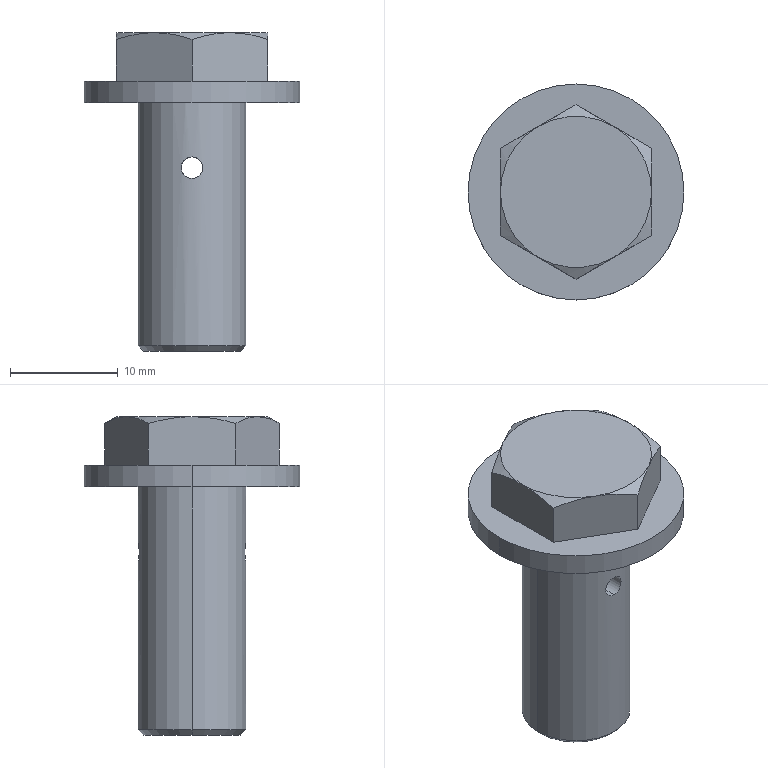Part | SolidWorks | features BaseBody 1 | 1 solid | 31 faces | box 20 x 20 x 29.5 mm | volume 2987 mm3 | plane 11 | cylinder 10 | cone 10 | commonest cylinder face diameters 2 x4 3.5 x2 10 x2 20 x2
STEP:
#1=CARTESIAN_POINT('',(135.5,59.,62.5));
#2=VERTEX_POINT('',#1);
#3=CARTESIAN_POINT('',(155.5,59.,62.5));
#4=VERTEX_POINT('',#3);
#5=CARTESIAN_POINT('',(145.5,59.,62.5));
#6=DIRECTION('',(0.,0.,-1.));
#7=DIRECTION('',(-1.,0.,0.));
#8=AXIS2_PLACEMENT_3D('',#5,#6,#7);
#9=CIRCLE('',#8,10.);
#10=EDGE_CURVE('',#2,#4,#9,.T.);
#11=ORIENTED_EDGE('',*,*,#10,.T.);
#12=CARTESIAN_POINT('',(155.5,59.,60.5));
#13=VERTEX_POINT('',#12);
#14=CARTESIAN_POINT('',(155.5,59.,62.5));
#15=DIRECTION('',(0.,0.,-1.));
#16=VECTOR('',#15,1000.);
#17=LINE('',#14,#16);
#18=EDGE_CURVE('',#4,#13,#17,.T.);
#19=ORIENTED_EDGE('',*,*,#18,.T.);
#20=CARTESIAN_POINT('',(135.5,59.,60.5));
#21=VERTEX_POINT('',#20);
#22=CARTESIAN_POINT('',(145.5,59.,60.5));
#23=DIRECTION('',(0.,0.,-1.));
#24=DIRECTION('',(-1.,0.,0.));
#25=AXIS2_PLACEMENT_3D('',#22,#23,#24);
#26=CIRCLE('',#25,10.);
#27=EDGE_CURVE('',#21,#13,#26,.T.);
#28=ORIENTED_EDGE('',*,*,#27,.F.);
#29=CARTESIAN_POINT('',(135.5,59.,62.5));
#30=DIRECTION('',(0.,0.,-1.));
#31=VECTOR('',#30,1000.);
#32=LINE('',#29,#31);
#33=EDGE_CURVE('',#2,#21,#32,.T.);
#34=ORIENTED_EDGE('',*,*,#33,.F.);
#35=EDGE_LOOP('',(#11,#19,#28,#34));
#36=FACE_OUTER_BOUND('',#35,.T.);
#37=CARTESIAN_POINT('',(145.5,59.,62.5));
#38=DIRECTION('',(0.,0.,-1.));
#39=DIRECTION('',(-1.,0.,0.));
#40=AXIS2_PLACEMENT_3D('',#37,#38,#39);
#41=CYLINDRICAL_SURFACE('',#40,10.);
#42=ADVANCED_FACE('',(#36),#41,.T.);
#43=CARTESIAN_POINT('',(145.5,54.,55.5));
#44=VERTEX_POINT('',#43);
#45=CARTESIAN_POINT('',(145.5,54.,53.5));
#46=VERTEX_POINT('',#45);
#47=CARTESIAN_POINT('',(145.5,54.,55.5));
#48=CARTESIAN_POINT('',(145.631,54.,55.5));
#49=CARTESIAN_POINT('',(145.763,54.005,55.474));
#50=CARTESIAN_POINT('',(146.003,54.024,55.374));
#51=CARTESIAN_POINT('',(146.114,54.037,55.3));
#52=CARTESIAN_POINT('',(146.299,54.063,55.115));
#53=CARTESIAN_POINT('',(146.373,54.077,55.005));
#54=CARTESIAN_POINT('',(146.474,54.095,54.763));
#55=CARTESIAN_POINT('',(146.5,54.101,54.633));
#56=CARTESIAN_POINT('',(146.5,54.101,54.368));
#57=CARTESIAN_POINT('',(146.474,54.095,54.238));
#58=CARTESIAN_POINT('',(146.374,54.077,53.996));
#59=CARTESIAN_POINT('',(146.299,54.063,53.885));
#60=CARTESIAN_POINT('',(146.116,54.037,53.701));
#61=CARTESIAN_POINT('',(146.004,54.024,53.627));
#62=CARTESIAN_POINT('',(145.764,54.006,53.527));
#63=CARTESIAN_POINT('',(145.632,54.,53.5));
#64=CARTESIAN_POINT('',(145.5,54.,53.5));
#65=B_SPLINE_CURVE_WITH_KNOTS('',3,(#47,#48,#49,#50,#51,#52,#53,#54,#55,#56,#57,#58,#59,#60,#61,#62,#63,#64),.UNSPECIFIED.,.F.,.F.,(4,2,2,2,2,2,2,2,4),(0.003134,0.003526,0.003918,0.004309,0.004701,0.005093,0.005485,0.005876,0.006268),.UNSPECIFIED.);
#66=EDGE_CURVE('',#44,#46,#65,.T.);
#67=ORIENTED_EDGE('',*,*,#66,.F.);
#68=CARTESIAN_POINT('',(145.5,57.25,55.5));
#69=VERTEX_POINT('',#68);
#70=CARTESIAN_POINT('',(145.5,50.917,55.5));
#71=DIRECTION('',(0.,1.,0.));
#72=VECTOR('',#71,1000.);
#73=LINE('',#70,#72);
#74=EDGE_CURVE('',#44,#69,#73,.T.);
#75=ORIENTED_EDGE('',*,*,#74,.T.);
#76=CARTESIAN_POINT('',(145.5,57.25,53.5));
#77=VERTEX_POINT('',#76);
#78=CARTESIAN_POINT('',(145.5,57.25,53.5));
#79=CARTESIAN_POINT('',(145.635,57.25,53.5));
#80=CARTESIAN_POINT('',(145.768,57.266,53.528));
#81=CARTESIAN_POINT('',(146.009,57.321,53.63));
#82=CARTESIAN_POINT('',(146.118,57.36,53.704));
#83=CARTESIAN_POINT('',(146.298,57.44,53.884));
#84=CARTESIAN_POINT('',(146.371,57.481,53.992));
#85=CARTESIAN_POINT('',(146.472,57.543,54.231));
#86=CARTESIAN_POINT('',(146.5,57.564,54.364));
#87=CARTESIAN_POINT('',(146.5,57.564,54.635));
#88=CARTESIAN_POINT('',(146.472,57.544,54.768));
#89=CARTESIAN_POINT('',(146.371,57.481,55.008));
#90=CARTESIAN_POINT('',(146.298,57.439,55.116));
#91=CARTESIAN_POINT('',(146.117,57.36,55.297));
#92=CARTESIAN_POINT('',(146.009,57.321,55.37));
#93=CARTESIAN_POINT('',(145.767,57.266,55.472));
#94=CARTESIAN_POINT('',(145.636,57.25,55.5));
#95=CARTESIAN_POINT('',(145.5,57.25,55.5));
#96=B_SPLINE_CURVE_WITH_KNOTS('',3,(#78,#79,#80,#81,#82,#83,#84,#85,#86,#87,#88,#89,#90,#91,#92,#93,#94,#95),.UNSPECIFIED.,.F.,.F.,(4,2,2,2,2,2,2,2,4),(0.,0.0003999,0.0007999,0.0012,0.0016,0.002,0.0024,0.0028,0.003199),.UNSPECIFIED.);
#97=EDGE_CURVE('',#77,#69,#96,.T.);
#98=ORIENTED_EDGE('',*,*,#97,.F.);
#99=CARTESIAN_POINT('',(145.5,50.917,53.5));
#100=DIRECTION('',(0.,1.,0.));
#101=VECTOR('',#100,1000.);
#102=LINE('',#99,#101);
#103=EDGE_CURVE('',#46,#77,#102,.T.);
#104=ORIENTED_EDGE('',*,*,#103,.F.);
#105=EDGE_LOOP('',(#67,#75,#98,#104));
#106=FACE_OUTER_BOUND('',#105,.T.);
#107=CARTESIAN_POINT('',(145.5,50.917,54.5));
#108=DIRECTION('',(0.,1.,0.));
#109=DIRECTION('',(0.,0.,-1.));
#110=AXIS2_PLACEMENT_3D('',#107,#108,#109);
#111=CYLINDRICAL_SURFACE('',#110,1.);
#112=ADVANCED_FACE('',(#106),#111,.F.);
#113=CARTESIAN_POINT('',(145.5,60.75,55.5));
#114=VERTEX_POINT('',#113);
#115=CARTESIAN_POINT('',(145.5,60.75,53.5));
#116=VERTEX_POINT('',#115);
#117=CARTESIAN_POINT('',(145.5,60.75,55.5));
#118=CARTESIAN_POINT('',(145.635,60.75,55.5));
#119=CARTESIAN_POINT('',(145.768,60.734,55.472));
#120=CARTESIAN_POINT('',(146.009,60.679,55.371));
#121=CARTESIAN_POINT('',(146.118,60.64,55.297));
#122=CARTESIAN_POINT('',(146.298,60.561,55.116));
#123=CARTESIAN_POINT('',(146.371,60.519,55.008));
#124=CARTESIAN_POINT('',(146.472,60.457,54.769));
#125=CARTESIAN_POINT('',(146.5,60.436,54.635));
#126=CARTESIAN_POINT('',(146.5,60.436,54.366));
#127=CARTESIAN_POINT('',(146.472,60.456,54.233));
#128=CARTESIAN_POINT('',(146.372,60.519,53.993));
#129=CARTESIAN_POINT('',(146.299,60.56,53.885));
#130=CARTESIAN_POINT('',(146.118,60.64,53.703));
#131=CARTESIAN_POINT('',(146.011,60.678,53.63));
#132=CARTESIAN_POINT('',(145.768,60.734,53.528));
#133=CARTESIAN_POINT('',(145.635,60.75,53.5));
#134=CARTESIAN_POINT('',(145.5,60.75,53.5));
#135=B_SPLINE_CURVE_WITH_KNOTS('',3,(#117,#118,#119,#120,#121,#122,#123,#124,#125,#126,#127,#128,#129,#130,#131,#132,#133,#134),.UNSPECIFIED.,.F.,.F.,(4,2,2,2,2,2,2,2,4),(0.003199,0.003599,0.003998,0.004397,0.004796,0.005195,0.005594,0.005993,0.006392),.UNSPECIFIED.);
#136=EDGE_CURVE('',#114,#116,#135,.T.);
#137=ORIENTED_EDGE('',*,*,#136,.F.);
#138=CARTESIAN_POINT('',(145.5,64.,55.5));
#139=VERTEX_POINT('',#138);
#140=CARTESIAN_POINT('',(145.5,50.917,55.5));
#141=DIRECTION('',(0.,1.,0.));
#142=VECTOR('',#141,1000.);
#143=LINE('',#140,#142);
#144=EDGE_CURVE('',#114,#139,#143,.T.);
#145=ORIENTED_EDGE('',*,*,#144,.T.);
#146=CARTESIAN_POINT('',(145.5,64.,53.5));
#147=VERTEX_POINT('',#146);
#148=CARTESIAN_POINT('',(145.5,64.,53.5));
#149=CARTESIAN_POINT('',(145.633,64.,53.5));
#150=CARTESIAN_POINT('',(145.763,63.995,53.526));
#151=CARTESIAN_POINT('',(146.005,63.976,53.627));
#152=CARTESIAN_POINT('',(146.115,63.963,53.701));
#153=CARTESIAN_POINT('',(146.299,63.937,53.885));
#154=CARTESIAN_POINT('',(146.374,63.923,53.996));
#155=CARTESIAN_POINT('',(146.474,63.905,54.237));
#156=CARTESIAN_POINT('',(146.5,63.899,54.369));
#157=CARTESIAN_POINT('',(146.5,63.899,54.63));
#158=CARTESIAN_POINT('',(146.474,63.904,54.762));
#159=CARTESIAN_POINT('',(146.374,63.923,55.004));
#160=CARTESIAN_POINT('',(146.3,63.936,55.114));
#161=CARTESIAN_POINT('',(146.114,63.963,55.3));
#162=CARTESIAN_POINT('',(146.004,63.976,55.374));
#163=CARTESIAN_POINT('',(145.762,63.995,55.474));
#164=CARTESIAN_POINT('',(145.631,64.,55.5));
#165=CARTESIAN_POINT('',(145.5,64.,55.5));
#166=B_SPLINE_CURVE_WITH_KNOTS('',3,(#148,#149,#150,#151,#152,#153,#154,#155,#156,#157,#158,#159,#160,#161,#162,#163,#164,#165),.UNSPECIFIED.,.F.,.F.,(4,2,2,2,2,2,2,2,4),(0.,0.0003918,0.0007836,0.001175,0.001567,0.001959,0.002351,0.002743,0.003134),.UNSPECIFIED.);
#167=EDGE_CURVE('',#147,#139,#166,.T.);
#168=ORIENTED_EDGE('',*,*,#167,.F.);
#169=CARTESIAN_POINT('',(145.5,50.917,53.5));
#170=DIRECTION('',(0.,1.,0.));
#171=VECTOR('',#170,1000.);
#172=LINE('',#169,#171);
#173=EDGE_CURVE('',#116,#147,#172,.T.);
#174=ORIENTED_EDGE('',*,*,#173,.F.);
#175=EDGE_LOOP('',(#137,#145,#168,#174));
#176=FACE_OUTER_BOUND('',#175,.T.);
#177=CARTESIAN_POINT('',(145.5,50.917,54.5));
#178=DIRECTION('',(0.,1.,0.));
#179=DIRECTION('',(0.,0.,-1.));
#180=AXIS2_PLACEMENT_3D('',#177,#178,#179);
#181=CYLINDRICAL_SURFACE('',#180,1.);
#182=ADVANCED_FACE('',(#176),#181,.F.);
#183=CARTESIAN_POINT('',(147.25,59.,38.));
#184=VERTEX_POINT('',#183);
#185=CARTESIAN_POINT('',(143.75,59.,38.));
#186=VERTEX_POINT('',#185);
#187=CARTESIAN_POINT('',(145.5,59.,38.));
#188=DIRECTION('',(0.,0.,-1.));
#189=DIRECTION('',(-1.,0.,0.));
#190=AXIS2_PLACEMENT_3D('',#187,#188,#189);
#191=CIRCLE('',#190,1.75);
#192=EDGE_CURVE('',#184,#186,#191,.T.);
#193=ORIENTED_EDGE('',*,*,#192,.F.);
#194=CARTESIAN_POINT('',(147.75,59.,37.5));
#195=VERTEX_POINT('',#194);
#196=CARTESIAN_POINT('',(147.25,59.,38.));
#197=DIRECTION('',(0.7071,0.,-0.7071));
#198=VECTOR('',#197,1000.);
#199=LINE('',#196,#198);
#200=EDGE_CURVE('',#184,#195,#199,.T.);
#201=ORIENTED_EDGE('',*,*,#200,.T.);
#202=CARTESIAN_POINT('',(143.25,59.,37.5));
#203=VERTEX_POINT('',#202);
#204=CARTESIAN_POINT('',(145.5,59.,37.5));
#205=DIRECTION('',(0.,0.,1.));
#206=DIRECTION('',(-1.,0.,0.));
#207=AXIS2_PLACEMENT_3D('',#204,#205,#206);
#208=CIRCLE('',#207,2.25);
#209=EDGE_CURVE('',#203,#195,#208,.T.);
#210=ORIENTED_EDGE('',*,*,#209,.F.);
#211=CARTESIAN_POINT('',(143.75,59.,38.));
#212=DIRECTION('',(-0.7071,0.,-0.7071));
#213=VECTOR('',#212,1000.);
#214=LINE('',#211,#213);
#215=EDGE_CURVE('',#186,#203,#214,.T.);
#216=ORIENTED_EDGE('',*,*,#215,.F.);
#217=EDGE_LOOP('',(#193,#201,#210,#216));
#218=FACE_OUTER_BOUND('',#217,.T.);
#219=CARTESIAN_POINT('',(145.5,59.,38.));
#220=DIRECTION('',(0.,0.,-1.));
#221=DIRECTION('',(-1.,0.,0.));
#222=AXIS2_PLACEMENT_3D('',#219,#220,#221);
#223=CONICAL_SURFACE('',#222,1.75,0.7854);
#224=ADVANCED_FACE('',(#218),#223,.F.);
#225=CARTESIAN_POINT('',(141.,59.,37.5));
#226=VERTEX_POINT('',#225);
#227=CARTESIAN_POINT('',(150.,59.,37.5));
#228=VERTEX_POINT('',#227);
#229=CARTESIAN_POINT('',(145.5,59.,37.5));
#230=DIRECTION('',(0.,0.,-1.));
#231=DIRECTION('',(-1.,0.,0.));
#232=AXIS2_PLACEMENT_3D('',#229,#230,#231);
#233=CIRCLE('',#232,4.5);
#234=EDGE_CURVE('',#226,#228,#233,.T.);
#235=ORIENTED_EDGE('',*,*,#234,.F.);
#236=CARTESIAN_POINT('',(140.5,59.,38.));
#237=VERTEX_POINT('',#236);
#238=CARTESIAN_POINT('',(141.,59.,37.5));
#239=DIRECTION('',(-0.7071,0.,0.7071));
#240=VECTOR('',#239,1000.);
#241=LINE('',#238,#240);
#242=EDGE_CURVE('',#226,#237,#241,.T.);
#243=ORIENTED_EDGE('',*,*,#242,.T.);
#244=CARTESIAN_POINT('',(150.5,59.,38.));
#245=VERTEX_POINT('',#244);
#246=CARTESIAN_POINT('',(145.5,59.,38.));
#247=DIRECTION('',(0.,0.,1.));
#248=DIRECTION('',(-1.,0.,0.));
#249=AXIS2_PLACEMENT_3D('',#246,#247,#248);
#250=CIRCLE('',#249,5.);
#251=EDGE_CURVE('',#245,#237,#250,.T.);
#252=ORIENTED_EDGE('',*,*,#251,.F.);
#253=CARTESIAN_POINT('',(150.,59.,37.5));
#254=DIRECTION('',(0.7071,0.,0.7071));
#255=VECTOR('',#254,1000.);
#256=LINE('',#253,#255);
#257=EDGE_CURVE('',#228,#245,#256,.T.);
#258=ORIENTED_EDGE('',*,*,#257,.F.);
#259=EDGE_LOOP('',(#235,#243,#252,#258));
#260=FACE_OUTER_BOUND('',#259,.T.);
#261=CARTESIAN_POINT('',(145.5,59.,37.5));
#262=DIRECTION('',(0.,0.,1.));
#263=DIRECTION('',(1.,0.,0.));
#264=AXIS2_PLACEMENT_3D('',#261,#262,#263);
#265=CONICAL_SURFACE('',#264,4.5,0.7854);
#266=ADVANCED_FACE('',(#260),#265,.T.);
#267=ORIENTED_EDGE('',*,*,#97,.T.);
#268=CARTESIAN_POINT('',(145.5,57.25,55.5));
#269=CARTESIAN_POINT('',(145.365,57.25,55.5));
#270=CARTESIAN_POINT('',(145.232,57.266,55.472));
#271=CARTESIAN_POINT('',(144.991,57.321,55.371));
#272=CARTESIAN_POINT('',(144.882,57.36,55.297));
#273=CARTESIAN_POINT('',(144.702,57.439,55.116));
#274=CARTESIAN_POINT('',(144.629,57.481,55.008));
#275=CARTESIAN_POINT('',(144.528,57.543,54.769));
#276=CARTESIAN_POINT('',(144.5,57.564,54.635));
#277=CARTESIAN_POINT('',(144.5,57.564,54.366));
#278=CARTESIAN_POINT('',(144.528,57.544,54.233));
#279=CARTESIAN_POINT('',(144.628,57.481,53.993));
#280=CARTESIAN_POINT('',(144.701,57.44,53.885));
#281=CARTESIAN_POINT('',(144.882,57.36,53.703));
#282=CARTESIAN_POINT('',(144.989,57.322,53.63));
#283=CARTESIAN_POINT('',(145.232,57.266,53.528));
#284=CARTESIAN_POINT('',(145.365,57.25,53.5));
#285=CARTESIAN_POINT('',(145.5,57.25,53.5));
#286=B_SPLINE_CURVE_WITH_KNOTS('',3,(#268,#269,#270,#271,#272,#273,#274,#275,#276,#277,#278,#279,#280,#281,#282,#283,#284,#285),.UNSPECIFIED.,.F.,.F.,(4,2,2,2,2,2,2,2,4),(0.003199,0.003599,0.003998,0.004397,0.004796,0.005195,0.005594,0.005993,0.006392),.UNSPECIFIED.);
#287=EDGE_CURVE('',#69,#77,#286,.T.);
#288=ORIENTED_EDGE('',*,*,#287,.T.);
#289=EDGE_LOOP('',(#267,#288));
#290=FACE_BOUND('',#289,.T.);
#291=CARTESIAN_POINT('',(147.25,59.,56.5));
#292=VERTEX_POINT('',#291);
#293=CARTESIAN_POINT('',(143.75,59.,56.5));
#294=VERTEX_POINT('',#293);
#295=CARTESIAN_POINT('',(145.5,59.,56.5));
#296=DIRECTION('',(0.,0.,-1.));
#297=DIRECTION('',(-1.,0.,0.));
#298=AXIS2_PLACEMENT_3D('',#295,#296,#297);
#299=CIRCLE('',#298,1.75);
#300=EDGE_CURVE('',#292,#294,#299,.T.);
#301=ORIENTED_EDGE('',*,*,#300,.F.);
#302=CARTESIAN_POINT('',(147.25,59.,56.5));
#303=DIRECTION('',(0.,0.,-1.));
#304=VECTOR('',#303,1000.);
#305=LINE('',#302,#304);
#306=EDGE_CURVE('',#292,#184,#305,.T.);
#307=ORIENTED_EDGE('',*,*,#306,.T.);
#308=ORIENTED_EDGE('',*,*,#192,.T.);
#309=CARTESIAN_POINT('',(143.75,59.,56.5));
#310=DIRECTION('',(0.,0.,-1.));
#311=VECTOR('',#310,1000.);
#312=LINE('',#309,#311);
#313=EDGE_CURVE('',#294,#186,#312,.T.);
#314=ORIENTED_EDGE('',*,*,#313,.F.);
#315=EDGE_LOOP('',(#301,#307,#308,#314));
#316=FACE_OUTER_BOUND('',#315,.T.);
#317=CARTESIAN_POINT('',(145.5,59.,56.5));
#318=DIRECTION('',(0.,0.,-1.));
#319=DIRECTION('',(-1.,0.,0.));
#320=AXIS2_PLACEMENT_3D('',#317,#318,#319);
#321=CYLINDRICAL_SURFACE('',#320,1.75);
#322=ADVANCED_FACE('',(#290,#316),#321,.F.);
#323=ORIENTED_EDGE('',*,*,#167,.T.);
#324=CARTESIAN_POINT('',(145.5,64.,55.5));
#325=CARTESIAN_POINT('',(145.369,64.,55.5));
#326=CARTESIAN_POINT('',(145.237,63.995,55.474));
#327=CARTESIAN_POINT('',(144.997,63.976,55.374));
#328=CARTESIAN_POINT('',(144.886,63.963,55.3));
#329=CARTESIAN_POINT('',(144.701,63.937,55.115));
#330=CARTESIAN_POINT('',(144.627,63.923,55.005));
#331=CARTESIAN_POINT('',(144.526,63.905,54.763));
#332=CARTESIAN_POINT('',(144.5,63.899,54.633));
#333=CARTESIAN_POINT('',(144.5,63.899,54.368));
#334=CARTESIAN_POINT('',(144.526,63.905,54.238));
#335=CARTESIAN_POINT('',(144.626,63.923,53.996));
#336=CARTESIAN_POINT('',(144.701,63.937,53.885));
#337=CARTESIAN_POINT('',(144.884,63.963,53.701));
#338=CARTESIAN_POINT('',(144.996,63.976,53.627));
#339=CARTESIAN_POINT('',(145.236,63.994,53.527));
#340=CARTESIAN_POINT('',(145.368,64.,53.5));
#341=CARTESIAN_POINT('',(145.5,64.,53.5));
#342=B_SPLINE_CURVE_WITH_KNOTS('',3,(#324,#325,#326,#327,#328,#329,#330,#331,#332,#333,#334,#335,#336,#337,#338,#339,#340,#341),.UNSPECIFIED.,.F.,.F.,(4,2,2,2,2,2,2,2,4),(0.003134,0.003526,0.003918,0.004309,0.004701,0.005093,0.005485,0.005876,0.006268),.UNSPECIFIED.);
#343=EDGE_CURVE('',#139,#147,#342,.T.);
#344=ORIENTED_EDGE('',*,*,#343,.T.);
#345=EDGE_LOOP('',(#323,#344));
#346=FACE_BOUND('',#345,.T.);
#347=ORIENTED_EDGE('',*,*,#251,.T.);
#348=CARTESIAN_POINT('',(140.5,59.,60.5));
#349=VERTEX_POINT('',#348);
#350=CARTESIAN_POINT('',(140.5,59.,37.5));
#351=DIRECTION('',(0.,0.,1.));
#352=VECTOR('',#351,1000.);
#353=LINE('',#350,#352);
#354=EDGE_CURVE('',#237,#349,#353,.T.);
#355=ORIENTED_EDGE('',*,*,#354,.T.);
#356=CARTESIAN_POINT('',(150.5,59.,60.5));
#357=VERTEX_POINT('',#356);
#358=CARTESIAN_POINT('',(145.5,59.,60.5));
#359=DIRECTION('',(0.,0.,-1.));
#360=DIRECTION('',(-1.,0.,0.));
#361=AXIS2_PLACEMENT_3D('',#358,#359,#360);
#362=CIRCLE('',#361,5.);
#363=EDGE_CURVE('',#349,#357,#362,.T.);
#364=ORIENTED_EDGE('',*,*,#363,.T.);
#365=CARTESIAN_POINT('',(150.5,59.,37.5));
#366=DIRECTION('',(0.,0.,1.));
#367=VECTOR('',#366,1000.);
#368=LINE('',#365,#367);
#369=EDGE_CURVE('',#245,#357,#368,.T.);
#370=ORIENTED_EDGE('',*,*,#369,.F.);
#371=EDGE_LOOP('',(#347,#355,#364,#370));
#372=FACE_OUTER_BOUND('',#371,.T.);
#373=CARTESIAN_POINT('',(145.5,59.,37.5));
#374=DIRECTION('',(0.,0.,1.));
#375=DIRECTION('',(1.,0.,0.));
#376=AXIS2_PLACEMENT_3D('',#373,#374,#375);
#377=CYLINDRICAL_SURFACE('',#376,5.);
#378=ADVANCED_FACE('',(#346,#372),#377,.T.);
#379=CARTESIAN_POINT('',(145.5,59.,60.5));
#380=DIRECTION('',(0.,0.,-1.));
#381=DIRECTION('',(-1.,0.,0.));
#382=AXIS2_PLACEMENT_3D('',#379,#380,#381);
#383=CIRCLE('',#382,5.);
#384=EDGE_CURVE('',#357,#349,#383,.T.);
#385=ORIENTED_EDGE('',*,*,#384,.F.);
#386=ORIENTED_EDGE('',*,*,#363,.F.);
#387=EDGE_LOOP('',(#385,#386));
#388=FACE_BOUND('',#387,.T.);
#389=ORIENTED_EDGE('',*,*,#27,.T.);
#390=CARTESIAN_POINT('',(145.5,59.,60.5));
#391=DIRECTION('',(0.,0.,-1.));
#392=DIRECTION('',(-1.,0.,0.));
#393=AXIS2_PLACEMENT_3D('',#390,#391,#392);
#394=CIRCLE('',#393,10.);
#395=EDGE_CURVE('',#13,#21,#394,.T.);
#396=ORIENTED_EDGE('',*,*,#395,.T.);
#397=EDGE_LOOP('',(#389,#396));
#398=FACE_OUTER_BOUND('',#397,.T.);
#399=CARTESIAN_POINT('',(145.5,67.083,60.5));
#400=DIRECTION('',(0.,0.,-1.));
#401=DIRECTION('',(-1.,0.,0.));
#402=AXIS2_PLACEMENT_3D('',#399,#400,#401);
#403=PLANE('',#402);
#404=ADVANCED_FACE('',(#388,#398),#403,.T.);
#405=ORIENTED_EDGE('',*,*,#354,.F.);
#406=CARTESIAN_POINT('',(145.5,59.,38.));
#407=DIRECTION('',(0.,0.,1.));
#408=DIRECTION('',(-1.,0.,0.));
#409=AXIS2_PLACEMENT_3D('',#406,#407,#408);
#410=CIRCLE('',#409,5.);
#411=EDGE_CURVE('',#237,#245,#410,.T.);
#412=ORIENTED_EDGE('',*,*,#411,.T.);
#413=ORIENTED_EDGE('',*,*,#369,.T.);
#414=ORIENTED_EDGE('',*,*,#384,.T.);
#415=EDGE_LOOP('',(#405,#412,#413,#414));
#416=FACE_OUTER_BOUND('',#415,.T.);
#417=CARTESIAN_POINT('',(145.5,54.,53.5));
#418=CARTESIAN_POINT('',(145.367,54.,53.5));
#419=CARTESIAN_POINT('',(145.237,54.005,53.526));
#420=CARTESIAN_POINT('',(144.995,54.024,53.627));
#421=CARTESIAN_POINT('',(144.885,54.037,53.701));
#422=CARTESIAN_POINT('',(144.701,54.063,53.885));
#423=CARTESIAN_POINT('',(144.626,54.077,53.996));
#424=CARTESIAN_POINT('',(144.526,54.095,54.237));
#425=CARTESIAN_POINT('',(144.5,54.101,54.369));
#426=CARTESIAN_POINT('',(144.5,54.101,54.63));
#427=CARTESIAN_POINT('',(144.526,54.096,54.762));
#428=CARTESIAN_POINT('',(144.626,54.077,55.004));
#429=CARTESIAN_POINT('',(144.7,54.064,55.114));
#430=CARTESIAN_POINT('',(144.886,54.037,55.3));
#431=CARTESIAN_POINT('',(144.996,54.024,55.374));
#432=CARTESIAN_POINT('',(145.238,54.005,55.474));
#433=CARTESIAN_POINT('',(145.369,54.,55.5));
#434=CARTESIAN_POINT('',(145.5,54.,55.5));
#435=B_SPLINE_CURVE_WITH_KNOTS('',3,(#417,#418,#419,#420,#421,#422,#423,#424,#425,#426,#427,#428,#429,#430,#431,#432,#433,#434),.UNSPECIFIED.,.F.,.F.,(4,2,2,2,2,2,2,2,4),(0.,0.0003918,0.0007836,0.001175,0.001567,0.001959,0.002351,0.002743,0.003134),.UNSPECIFIED.);
#436=EDGE_CURVE('',#46,#44,#435,.T.);
#437=ORIENTED_EDGE('',*,*,#436,.T.);
#438=ORIENTED_EDGE('',*,*,#66,.T.);
#439=EDGE_LOOP('',(#437,#438));
#440=FACE_BOUND('',#439,.T.);
#441=CARTESIAN_POINT('',(145.5,59.,37.5));
#442=DIRECTION('',(0.,0.,1.));
#443=DIRECTION('',(1.,0.,0.));
#444=AXIS2_PLACEMENT_3D('',#441,#442,#443);
#445=CYLINDRICAL_SURFACE('',#444,5.);
#446=ADVANCED_FACE('',(#416,#440),#445,.T.);
#447=ORIENTED_EDGE('',*,*,#209,.T.);
#448=CARTESIAN_POINT('',(145.5,59.,37.5));
#449=DIRECTION('',(0.,0.,1.));
#450=DIRECTION('',(-1.,0.,0.));
#451=AXIS2_PLACEMENT_3D('',#448,#449,#450);
#452=CIRCLE('',#451,2.25);
#453=EDGE_CURVE('',#195,#203,#452,.T.);
#454=ORIENTED_EDGE('',*,*,#453,.T.);
#455=EDGE_LOOP('',(#447,#454));
#456=FACE_BOUND('',#455,.T.);
#457=CARTESIAN_POINT('',(145.5,59.,37.5));
#458=DIRECTION('',(0.,0.,-1.));
#459=DIRECTION('',(-1.,0.,0.));
#460=AXIS2_PLACEMENT_3D('',#457,#458,#459);
#461=CIRCLE('',#460,4.5);
#462=EDGE_CURVE('',#228,#226,#461,.T.);
#463=ORIENTED_EDGE('',*,*,#462,.T.);
#464=ORIENTED_EDGE('',*,*,#234,.T.);
#465=EDGE_LOOP('',(#463,#464));
#466=FACE_OUTER_BOUND('',#465,.T.);
#467=CARTESIAN_POINT('',(145.5,59.,37.5));
#468=DIRECTION('',(0.,0.,-1.));
#469=DIRECTION('',(-1.,0.,0.));
#470=AXIS2_PLACEMENT_3D('',#467,#468,#469);
#471=PLANE('',#470);
#472=ADVANCED_FACE('',(#456,#466),#471,.T.);
#473=ORIENTED_EDGE('',*,*,#306,.F.);
#474=CARTESIAN_POINT('',(145.5,59.,56.5));
#475=DIRECTION('',(0.,0.,-1.));
#476=DIRECTION('',(-1.,0.,0.));
#477=AXIS2_PLACEMENT_3D('',#474,#475,#476);
#478=CIRCLE('',#477,1.75);
#479=EDGE_CURVE('',#294,#292,#478,.T.);
#480=ORIENTED_EDGE('',*,*,#479,.F.);
#481=ORIENTED_EDGE('',*,*,#313,.T.);
#482=CARTESIAN_POINT('',(145.5,59.,38.));
#483=DIRECTION('',(0.,0.,-1.));
#484=DIRECTION('',(-1.,0.,0.));
#485=AXIS2_PLACEMENT_3D('',#482,#483,#484);
#486=CIRCLE('',#485,1.75);
#487=EDGE_CURVE('',#186,#184,#486,.T.);
#488=ORIENTED_EDGE('',*,*,#487,.T.);
#489=EDGE_LOOP('',(#473,#480,#481,#488));
#490=FACE_OUTER_BOUND('',#489,.T.);
#491=CARTESIAN_POINT('',(145.5,60.75,53.5));
#492=CARTESIAN_POINT('',(145.365,60.75,53.5));
#493=CARTESIAN_POINT('',(145.232,60.734,53.528));
#494=CARTESIAN_POINT('',(144.991,60.679,53.63));
#495=CARTESIAN_POINT('',(144.882,60.64,53.704));
#496=CARTESIAN_POINT('',(144.702,60.56,53.884));
#497=CARTESIAN_POINT('',(144.629,60.519,53.992));
#498=CARTESIAN_POINT('',(144.528,60.457,54.231));
#499=CARTESIAN_POINT('',(144.5,60.436,54.364));
#500=CARTESIAN_POINT('',(144.5,60.436,54.635));
#501=CARTESIAN_POINT('',(144.528,60.456,54.768));
#502=CARTESIAN_POINT('',(144.629,60.519,55.008));
#503=CARTESIAN_POINT('',(144.702,60.561,55.116));
#504=CARTESIAN_POINT('',(144.883,60.64,55.297));
#505=CARTESIAN_POINT('',(144.991,60.679,55.37));
#506=CARTESIAN_POINT('',(145.233,60.734,55.472));
#507=CARTESIAN_POINT('',(145.364,60.75,55.5));
#508=CARTESIAN_POINT('',(145.5,60.75,55.5));
#509=B_SPLINE_CURVE_WITH_KNOTS('',3,(#491,#492,#493,#494,#495,#496,#497,#498,#499,#500,#501,#502,#503,#504,#505,#506,#507,#508),.UNSPECIFIED.,.F.,.F.,(4,2,2,2,2,2,2,2,4),(0.,0.0003999,0.0007999,0.0012,0.0016,0.002,0.0024,0.0028,0.003199),.UNSPECIFIED.);
#510=EDGE_CURVE('',#116,#114,#509,.T.);
#511=ORIENTED_EDGE('',*,*,#510,.T.);
#512=ORIENTED_EDGE('',*,*,#136,.T.);
#513=EDGE_LOOP('',(#511,#512));
#514=FACE_BOUND('',#513,.T.);
#515=CARTESIAN_POINT('',(145.5,59.,56.5));
#516=DIRECTION('',(0.,0.,-1.));
#517=DIRECTION('',(-1.,0.,0.));
#518=AXIS2_PLACEMENT_3D('',#515,#516,#517);
#519=CYLINDRICAL_SURFACE('',#518,1.75);
#520=ADVANCED_FACE('',(#490,#514),#519,.F.);
#521=ORIENTED_EDGE('',*,*,#479,.T.);
#522=ORIENTED_EDGE('',*,*,#300,.T.);
#523=EDGE_LOOP('',(#521,#522));
#524=FACE_OUTER_BOUND('',#523,.T.);
#525=CARTESIAN_POINT('',(145.5,59.,56.5));
#526=DIRECTION('',(0.,0.,-1.));
#527=DIRECTION('',(-1.,0.,0.));
#528=AXIS2_PLACEMENT_3D('',#525,#526,#527);
#529=PLANE('',#528);
#530=ADVANCED_FACE('',(#524),#529,.T.);
#531=ORIENTED_EDGE('',*,*,#242,.F.);
#532=ORIENTED_EDGE('',*,*,#462,.F.);
#533=ORIENTED_EDGE('',*,*,#257,.T.);
#534=ORIENTED_EDGE('',*,*,#411,.F.);
#535=EDGE_LOOP('',(#531,#532,#533,#534));
#536=FACE_OUTER_BOUND('',#535,.T.);
#537=CARTESIAN_POINT('',(145.5,59.,37.5));
#538=DIRECTION('',(0.,0.,1.));
#539=DIRECTION('',(1.,0.,0.));
#540=AXIS2_PLACEMENT_3D('',#537,#538,#539);
#541=CONICAL_SURFACE('',#540,4.5,0.7854);
#542=ADVANCED_FACE('',(#536),#541,.T.);
#543=ORIENTED_EDGE('',*,*,#200,.F.);
#544=ORIENTED_EDGE('',*,*,#487,.F.);
#545=ORIENTED_EDGE('',*,*,#215,.T.);
#546=ORIENTED_EDGE('',*,*,#453,.F.);
#547=EDGE_LOOP('',(#543,#544,#545,#546));
#548=FACE_OUTER_BOUND('',#547,.T.);
#549=CARTESIAN_POINT('',(145.5,59.,38.));
#550=DIRECTION('',(0.,0.,-1.));
#551=DIRECTION('',(-1.,0.,0.));
#552=AXIS2_PLACEMENT_3D('',#549,#550,#551);
#553=CONICAL_SURFACE('',#552,1.75,0.7854);
#554=ADVANCED_FACE('',(#548),#553,.F.);
#555=ORIENTED_EDGE('',*,*,#144,.F.);
#556=ORIENTED_EDGE('',*,*,#510,.F.);
#557=ORIENTED_EDGE('',*,*,#173,.T.);
#558=ORIENTED_EDGE('',*,*,#343,.F.);
#559=EDGE_LOOP('',(#555,#556,#557,#558));
#560=FACE_OUTER_BOUND('',#559,.T.);
#561=CARTESIAN_POINT('',(145.5,50.917,54.5));
#562=DIRECTION('',(0.,1.,0.));
#563=DIRECTION('',(0.,0.,-1.));
#564=AXIS2_PLACEMENT_3D('',#561,#562,#563);
#565=CYLINDRICAL_SURFACE('',#564,1.);
#566=ADVANCED_FACE('',(#560),#565,.F.);
#567=ORIENTED_EDGE('',*,*,#74,.F.);
#568=ORIENTED_EDGE('',*,*,#436,.F.);
#569=ORIENTED_EDGE('',*,*,#103,.T.);
#570=ORIENTED_EDGE('',*,*,#287,.F.);
#571=EDGE_LOOP('',(#567,#568,#569,#570));
#572=FACE_OUTER_BOUND('',#571,.T.);
#573=CARTESIAN_POINT('',(145.5,50.917,54.5));
#574=DIRECTION('',(0.,1.,0.));
#575=DIRECTION('',(0.,0.,-1.));
#576=AXIS2_PLACEMENT_3D('',#573,#574,#575);
#577=CYLINDRICAL_SURFACE('',#576,1.);
#578=ADVANCED_FACE('',(#572),#577,.F.);
#579=ORIENTED_EDGE('',*,*,#10,.F.);
#580=CARTESIAN_POINT('',(145.5,59.,62.5));
#581=DIRECTION('',(0.,0.,-1.));
#582=DIRECTION('',(-1.,0.,0.));
#583=AXIS2_PLACEMENT_3D('',#580,#581,#582);
#584=CIRCLE('',#583,10.);
#585=EDGE_CURVE('',#4,#2,#584,.T.);
#586=ORIENTED_EDGE('',*,*,#585,.F.);
#587=EDGE_LOOP('',(#579,#586));
#588=FACE_OUTER_BOUND('',#587,.T.);
#589=CARTESIAN_POINT('',(138.5,63.041,62.5));
#590=VERTEX_POINT('',#589);
#591=CARTESIAN_POINT('',(145.5,67.083,62.5));
#592=VERTEX_POINT('',#591);
#593=CARTESIAN_POINT('',(145.5,67.083,62.5));
#594=DIRECTION('',(0.866,0.5,0.));
#595=VECTOR('',#594,1000.);
#596=LINE('',#593,#595);
#597=EDGE_CURVE('',#590,#592,#596,.T.);
#598=ORIENTED_EDGE('',*,*,#597,.T.);
#599=CARTESIAN_POINT('',(152.5,63.041,62.5));
#600=VERTEX_POINT('',#599);
#601=CARTESIAN_POINT('',(145.5,67.083,62.5));
#602=DIRECTION('',(0.866,-0.5,0.));
#603=VECTOR('',#602,1000.);
#604=LINE('',#601,#603);
#605=EDGE_CURVE('',#592,#600,#604,.T.);
#606=ORIENTED_EDGE('',*,*,#605,.T.);
#607=CARTESIAN_POINT('',(152.5,54.959,62.5));
#608=VERTEX_POINT('',#607);
#609=CARTESIAN_POINT('',(152.5,54.959,62.5));
#610=DIRECTION('',(0.,-1.,0.));
#611=VECTOR('',#610,1000.);
#612=LINE('',#609,#611);
#613=EDGE_CURVE('',#600,#608,#612,.T.);
#614=ORIENTED_EDGE('',*,*,#613,.T.);
#615=CARTESIAN_POINT('',(145.5,50.917,62.5));
#616=VERTEX_POINT('',#615);
#617=CARTESIAN_POINT('',(145.5,50.917,62.5));
#618=DIRECTION('',(-0.866,-0.5,0.));
#619=VECTOR('',#618,1000.);
#620=LINE('',#617,#619);
#621=EDGE_CURVE('',#608,#616,#620,.T.);
#622=ORIENTED_EDGE('',*,*,#621,.T.);
#623=CARTESIAN_POINT('',(138.5,54.959,62.5));
#624=VERTEX_POINT('',#623);
#625=CARTESIAN_POINT('',(145.5,50.917,62.5));
#626=DIRECTION('',(-0.866,0.5,0.));
#627=VECTOR('',#626,1000.);
#628=LINE('',#625,#627);
#629=EDGE_CURVE('',#616,#624,#628,.T.);
#630=ORIENTED_EDGE('',*,*,#629,.T.);
#631=CARTESIAN_POINT('',(138.5,63.041,62.5));
#632=DIRECTION('',(0.,1.,0.));
#633=VECTOR('',#632,1000.);
#634=LINE('',#631,#633);
#635=EDGE_CURVE('',#624,#590,#634,.T.);
#636=ORIENTED_EDGE('',*,*,#635,.T.);
#637=EDGE_LOOP('',(#598,#606,#614,#622,#630,#636));
#638=FACE_BOUND('',#637,.T.);
#639=CARTESIAN_POINT('',(145.5,59.,62.5));
#640=DIRECTION('',(0.,0.,-1.));
#641=DIRECTION('',(-1.,0.,0.));
#642=AXIS2_PLACEMENT_3D('',#639,#640,#641);
#643=PLANE('',#642);
#644=ADVANCED_FACE('',(#588,#638),#643,.F.);
#645=ORIENTED_EDGE('',*,*,#18,.F.);
#646=ORIENTED_EDGE('',*,*,#585,.T.);
#647=ORIENTED_EDGE('',*,*,#33,.T.);
#648=ORIENTED_EDGE('',*,*,#395,.F.);
#649=EDGE_LOOP('',(#645,#646,#647,#648));
#650=FACE_OUTER_BOUND('',#649,.T.);
#651=CARTESIAN_POINT('',(145.5,59.,62.5));
#652=DIRECTION('',(0.,0.,-1.));
#653=DIRECTION('',(-1.,0.,0.));
#654=AXIS2_PLACEMENT_3D('',#651,#652,#653);
#655=CYLINDRICAL_SURFACE('',#654,10.);
#656=ADVANCED_FACE('',(#650),#655,.T.);
#657=CARTESIAN_POINT('',(149.,65.062,67.));
#658=VERTEX_POINT('',#657);
#659=CARTESIAN_POINT('',(142.,65.062,67.));
#660=VERTEX_POINT('',#659);
#661=CARTESIAN_POINT('',(145.5,59.,67.));
#662=DIRECTION('',(0.,0.,1.));
#663=DIRECTION('',(1.,0.,0.));
#664=AXIS2_PLACEMENT_3D('',#661,#662,#663);
#665=CIRCLE('',#664,7.);
#666=EDGE_CURVE('',#658,#660,#665,.T.);
#667=ORIENTED_EDGE('',*,*,#666,.T.);
#668=CARTESIAN_POINT('',(138.5,59.,67.));
#669=VERTEX_POINT('',#668);
#670=CARTESIAN_POINT('',(145.5,59.,67.));
#671=DIRECTION('',(0.,0.,1.));
#672=DIRECTION('',(1.,0.,0.));
#673=AXIS2_PLACEMENT_3D('',#670,#671,#672);
#674=CIRCLE('',#673,7.);
#675=EDGE_CURVE('',#660,#669,#674,.T.);
#676=ORIENTED_EDGE('',*,*,#675,.T.);
#677=CARTESIAN_POINT('',(142.,52.938,67.));
#678=VERTEX_POINT('',#677);
#679=CARTESIAN_POINT('',(145.5,59.,67.));
#680=DIRECTION('',(0.,0.,1.));
#681=DIRECTION('',(1.,0.,0.));
#682=AXIS2_PLACEMENT_3D('',#679,#680,#681);
#683=CIRCLE('',#682,7.);
#684=EDGE_CURVE('',#669,#678,#683,.T.);
#685=ORIENTED_EDGE('',*,*,#684,.T.);
#686=CARTESIAN_POINT('',(149.,52.938,67.));
#687=VERTEX_POINT('',#686);
#688=CARTESIAN_POINT('',(145.5,59.,67.));
#689=DIRECTION('',(0.,0.,1.));
#690=DIRECTION('',(1.,0.,0.));
#691=AXIS2_PLACEMENT_3D('',#688,#689,#690);
#692=CIRCLE('',#691,7.);
#693=EDGE_CURVE('',#678,#687,#692,.T.);
#694=ORIENTED_EDGE('',*,*,#693,.T.);
#695=CARTESIAN_POINT('',(152.5,59.,67.));
#696=VERTEX_POINT('',#695);
#697=CARTESIAN_POINT('',(145.5,59.,67.));
#698=DIRECTION('',(0.,0.,1.));
#699=DIRECTION('',(1.,0.,0.));
#700=AXIS2_PLACEMENT_3D('',#697,#698,#699);
#701=CIRCLE('',#700,7.);
#702=EDGE_CURVE('',#687,#696,#701,.T.);
#703=ORIENTED_EDGE('',*,*,#702,.T.);
#704=CARTESIAN_POINT('',(145.5,59.,67.));
#705=DIRECTION('',(0.,0.,1.));
#706=DIRECTION('',(1.,0.,0.));
#707=AXIS2_PLACEMENT_3D('',#704,#705,#706);
#708=CIRCLE('',#707,7.);
#709=EDGE_CURVE('',#696,#658,#708,.T.);
#710=ORIENTED_EDGE('',*,*,#709,.T.);
#711=EDGE_LOOP('',(#667,#676,#685,#694,#703,#710));
#712=FACE_OUTER_BOUND('',#711,.T.);
#713=CARTESIAN_POINT('',(145.5,67.083,67.));
#714=DIRECTION('',(0.,0.,-1.));
#715=DIRECTION('',(-1.,0.,0.));
#716=AXIS2_PLACEMENT_3D('',#713,#714,#715);
#717=PLANE('',#716);
#718=ADVANCED_FACE('',(#712),#717,.F.);
#719=CARTESIAN_POINT('',(152.5,63.041,66.375));
#720=VERTEX_POINT('',#719);
#721=CARTESIAN_POINT('',(149.,65.062,67.));
#722=CARTESIAN_POINT('',(149.297,64.891,67.));
#723=CARTESIAN_POINT('',(149.595,64.718,66.985));
#724=CARTESIAN_POINT('',(150.186,64.378,66.928));
#725=CARTESIAN_POINT('',(150.479,64.208,66.886));
#726=CARTESIAN_POINT('',(151.353,63.704,66.722));
#727=CARTESIAN_POINT('',(151.929,63.371,66.565));
#728=CARTESIAN_POINT('',(152.5,63.041,66.375));
#729=B_SPLINE_CURVE_WITH_KNOTS('',3,(#721,#722,#723,#724,#725,#726,#727,#728),.UNSPECIFIED.,.F.,.F.,(4,2,2,4),(0.00409,0.005108,0.006127,0.008164),.UNSPECIFIED.);
#730=EDGE_CURVE('',#658,#720,#729,.T.);
#731=ORIENTED_EDGE('',*,*,#730,.F.);
#732=ORIENTED_EDGE('',*,*,#709,.F.);
#733=CARTESIAN_POINT('',(152.5,63.041,66.375));
#734=CARTESIAN_POINT('',(152.5,62.388,66.563));
#735=CARTESIAN_POINT('',(152.5,61.726,66.721));
#736=CARTESIAN_POINT('',(152.5,60.377,66.94));
#737=CARTESIAN_POINT('',(152.5,59.684,67.));
#738=CARTESIAN_POINT('',(152.5,59.,67.));
#739=B_SPLINE_CURVE_WITH_KNOTS('',3,(#733,#734,#735,#736,#737,#738),.UNSPECIFIED.,.F.,.F.,(4,2,4),(0.02238,0.02443,0.02647),.UNSPECIFIED.);
#740=EDGE_CURVE('',#720,#696,#739,.T.);
#741=ORIENTED_EDGE('',*,*,#740,.F.);
#742=EDGE_LOOP('',(#731,#732,#741));
#743=FACE_OUTER_BOUND('',#742,.T.);
#744=CARTESIAN_POINT('',(145.5,59.,67.));
#745=DIRECTION('',(0.,0.,-1.));
#746=DIRECTION('',(1.,0.,0.));
#747=AXIS2_PLACEMENT_3D('',#744,#745,#746);
#748=CONICAL_SURFACE('',#747,7.,1.047);
#749=ADVANCED_FACE('',(#743),#748,.T.);
#750=CARTESIAN_POINT('',(152.5,54.959,66.375));
#751=VERTEX_POINT('',#750);
#752=CARTESIAN_POINT('',(152.5,59.,67.));
#753=CARTESIAN_POINT('',(152.5,58.317,67.));
#754=CARTESIAN_POINT('',(152.5,57.638,66.941));
#755=CARTESIAN_POINT('',(152.5,56.289,66.724));
#756=CARTESIAN_POINT('',(152.5,55.616,66.565));
#757=CARTESIAN_POINT('',(152.5,54.959,66.375));
#758=B_SPLINE_CURVE_WITH_KNOTS('',3,(#752,#753,#754,#755,#756,#757),.UNSPECIFIED.,.F.,.F.,(4,2,4),(0.02647,0.02852,0.03056),.UNSPECIFIED.);
#759=EDGE_CURVE('',#696,#751,#758,.T.);
#760=ORIENTED_EDGE('',*,*,#759,.F.);
#761=ORIENTED_EDGE('',*,*,#702,.F.);
#762=CARTESIAN_POINT('',(152.5,54.959,66.375));
#763=CARTESIAN_POINT('',(151.927,54.628,66.566));
#764=CARTESIAN_POINT('',(151.351,54.295,66.723));
#765=CARTESIAN_POINT('',(150.185,53.622,66.94));
#766=CARTESIAN_POINT('',(149.596,53.282,67.));
#767=CARTESIAN_POINT('',(149.,52.938,67.));
#768=B_SPLINE_CURVE_WITH_KNOTS('',3,(#762,#763,#764,#765,#766,#767),.UNSPECIFIED.,.F.,.F.,(4,2,4),(0.000000238,0.002045,0.00409),.UNSPECIFIED.);
#769=EDGE_CURVE('',#751,#687,#768,.T.);
#770=ORIENTED_EDGE('',*,*,#769,.F.);
#771=EDGE_LOOP('',(#760,#761,#770));
#772=FACE_OUTER_BOUND('',#771,.T.);
#773=CARTESIAN_POINT('',(145.5,59.,67.));
#774=DIRECTION('',(0.,0.,-1.));
#775=DIRECTION('',(1.,0.,0.));
#776=AXIS2_PLACEMENT_3D('',#773,#774,#775);
#777=CONICAL_SURFACE('',#776,7.,1.047);
#778=ADVANCED_FACE('',(#772),#777,.T.);
#779=CARTESIAN_POINT('',(145.5,50.917,66.375));
#780=VERTEX_POINT('',#779);
#781=CARTESIAN_POINT('',(149.,52.938,67.));
#782=CARTESIAN_POINT('',(148.703,52.766,67.));
#783=CARTESIAN_POINT('',(148.405,52.594,66.985));
#784=CARTESIAN_POINT('',(147.814,52.253,66.928));
#785=CARTESIAN_POINT('',(147.521,52.084,66.886));
#786=CARTESIAN_POINT('',(146.647,51.579,66.722));
#787=CARTESIAN_POINT('',(146.071,51.247,66.565));
#788=CARTESIAN_POINT('',(145.5,50.917,66.375));
#789=B_SPLINE_CURVE_WITH_KNOTS('',3,(#781,#782,#783,#784,#785,#786,#787,#788),.UNSPECIFIED.,.F.,.F.,(4,2,2,4),(0.00409,0.005108,0.006127,0.008164),.UNSPECIFIED.);
#790=EDGE_CURVE('',#687,#780,#789,.T.);
#791=ORIENTED_EDGE('',*,*,#790,.F.);
#792=ORIENTED_EDGE('',*,*,#693,.F.);
#793=CARTESIAN_POINT('',(145.5,50.917,66.375));
#794=CARTESIAN_POINT('',(144.927,51.248,66.566));
#795=CARTESIAN_POINT('',(144.351,51.581,66.723));
#796=CARTESIAN_POINT('',(143.185,52.254,66.94));
#797=CARTESIAN_POINT('',(142.596,52.594,67.));
#798=CARTESIAN_POINT('',(142.,52.938,67.));
#799=B_SPLINE_CURVE_WITH_KNOTS('',3,(#793,#794,#795,#796,#797,#798),.UNSPECIFIED.,.F.,.F.,(4,2,4),(0.000000238,0.002045,0.00409),.UNSPECIFIED.);
#800=EDGE_CURVE('',#780,#678,#799,.T.);
#801=ORIENTED_EDGE('',*,*,#800,.F.);
#802=EDGE_LOOP('',(#791,#792,#801));
#803=FACE_OUTER_BOUND('',#802,.T.);
#804=CARTESIAN_POINT('',(145.5,59.,67.));
#805=DIRECTION('',(0.,0.,-1.));
#806=DIRECTION('',(1.,0.,0.));
#807=AXIS2_PLACEMENT_3D('',#804,#805,#806);
#808=CONICAL_SURFACE('',#807,7.,1.047);
#809=ADVANCED_FACE('',(#803),#808,.T.);
#810=CARTESIAN_POINT('',(138.5,54.959,66.375));
#811=VERTEX_POINT('',#810);
#812=CARTESIAN_POINT('',(142.,52.938,67.));
#813=CARTESIAN_POINT('',(141.703,53.109,67.));
#814=CARTESIAN_POINT('',(141.405,53.282,66.985));
#815=CARTESIAN_POINT('',(140.814,53.622,66.928));
#816=CARTESIAN_POINT('',(140.521,53.792,66.886));
#817=CARTESIAN_POINT('',(139.647,54.296,66.722));
#818=CARTESIAN_POINT('',(139.071,54.629,66.565));
#819=CARTESIAN_POINT('',(138.5,54.959,66.375));
#820=B_SPLINE_CURVE_WITH_KNOTS('',3,(#812,#813,#814,#815,#816,#817,#818,#819),.UNSPECIFIED.,.F.,.F.,(4,2,2,4),(0.00409,0.005108,0.006127,0.008164),.UNSPECIFIED.);
#821=EDGE_CURVE('',#678,#811,#820,.T.);
#822=ORIENTED_EDGE('',*,*,#821,.F.);
#823=ORIENTED_EDGE('',*,*,#684,.F.);
#824=CARTESIAN_POINT('',(138.5,54.959,66.375));
#825=CARTESIAN_POINT('',(138.5,55.616,66.565));
#826=CARTESIAN_POINT('',(138.5,56.289,66.724));
#827=CARTESIAN_POINT('',(138.5,57.638,66.941));
#828=CARTESIAN_POINT('',(138.5,58.317,67.));
#829=CARTESIAN_POINT('',(138.5,59.,67.));
#830=B_SPLINE_CURVE_WITH_KNOTS('',3,(#824,#825,#826,#827,#828,#829),.UNSPECIFIED.,.F.,.F.,(4,2,4),(0.007365,0.00941,0.01146),.UNSPECIFIED.);
#831=EDGE_CURVE('',#811,#669,#830,.T.);
#832=ORIENTED_EDGE('',*,*,#831,.F.);
#833=EDGE_LOOP('',(#822,#823,#832));
#834=FACE_OUTER_BOUND('',#833,.T.);
#835=CARTESIAN_POINT('',(145.5,59.,67.));
#836=DIRECTION('',(0.,0.,-1.));
#837=DIRECTION('',(1.,0.,0.));
#838=AXIS2_PLACEMENT_3D('',#835,#836,#837);
#839=CONICAL_SURFACE('',#838,7.,1.047);
#840=ADVANCED_FACE('',(#834),#839,.T.);
#841=CARTESIAN_POINT('',(145.5,67.083,66.375));
#842=VERTEX_POINT('',#841);
#843=CARTESIAN_POINT('',(145.5,67.083,66.375));
#844=CARTESIAN_POINT('',(146.073,66.752,66.566));
#845=CARTESIAN_POINT('',(146.649,66.419,66.723));
#846=CARTESIAN_POINT('',(147.815,65.746,66.94));
#847=CARTESIAN_POINT('',(148.404,65.406,67.));
#848=CARTESIAN_POINT('',(149.,65.062,67.));
#849=B_SPLINE_CURVE_WITH_KNOTS('',3,(#843,#844,#845,#846,#847,#848),.UNSPECIFIED.,.F.,.F.,(4,2,4),(0.000000238,0.002045,0.00409),.UNSPECIFIED.);
#850=EDGE_CURVE('',#842,#658,#849,.T.);
#851=ORIENTED_EDGE('',*,*,#850,.F.);
#852=CARTESIAN_POINT('',(142.,65.062,67.));
#853=CARTESIAN_POINT('',(142.297,65.234,67.));
#854=CARTESIAN_POINT('',(142.595,65.406,66.985));
#855=CARTESIAN_POINT('',(143.186,65.747,66.928));
#856=CARTESIAN_POINT('',(143.479,65.916,66.886));
#857=CARTESIAN_POINT('',(144.353,66.421,66.722));
#858=CARTESIAN_POINT('',(144.929,66.753,66.565));
#859=CARTESIAN_POINT('',(145.5,67.083,66.375));
#860=B_SPLINE_CURVE_WITH_KNOTS('',3,(#852,#853,#854,#855,#856,#857,#858,#859),.UNSPECIFIED.,.F.,.F.,(4,2,2,4),(0.00409,0.005108,0.006127,0.008164),.UNSPECIFIED.);
#861=EDGE_CURVE('',#660,#842,#860,.T.);
#862=ORIENTED_EDGE('',*,*,#861,.F.);
#863=ORIENTED_EDGE('',*,*,#666,.F.);
#864=EDGE_LOOP('',(#851,#862,#863));
#865=FACE_OUTER_BOUND('',#864,.T.);
#866=CARTESIAN_POINT('',(145.5,59.,67.));
#867=DIRECTION('',(0.,0.,-1.));
#868=DIRECTION('',(1.,0.,0.));
#869=AXIS2_PLACEMENT_3D('',#866,#867,#868);
#870=CONICAL_SURFACE('',#869,7.,1.047);
#871=ADVANCED_FACE('',(#865),#870,.T.);
#872=CARTESIAN_POINT('',(138.5,63.041,66.375));
#873=VERTEX_POINT('',#872);
#874=CARTESIAN_POINT('',(138.5,59.,67.));
#875=CARTESIAN_POINT('',(138.5,59.684,67.));
#876=CARTESIAN_POINT('',(138.5,60.377,66.94));
#877=CARTESIAN_POINT('',(138.5,61.726,66.721));
#878=CARTESIAN_POINT('',(138.5,62.388,66.563));
#879=CARTESIAN_POINT('',(138.5,63.041,66.375));
#880=B_SPLINE_CURVE_WITH_KNOTS('',3,(#874,#875,#876,#877,#878,#879),.UNSPECIFIED.,.F.,.F.,(4,2,4),(0.01146,0.0135,0.01555),.UNSPECIFIED.);
#881=EDGE_CURVE('',#669,#873,#880,.T.);
#882=ORIENTED_EDGE('',*,*,#881,.F.);
#883=ORIENTED_EDGE('',*,*,#675,.F.);
#884=CARTESIAN_POINT('',(138.5,63.041,66.375));
#885=CARTESIAN_POINT('',(139.073,63.372,66.566));
#886=CARTESIAN_POINT('',(139.649,63.705,66.723));
#887=CARTESIAN_POINT('',(140.815,64.378,66.94));
#888=CARTESIAN_POINT('',(141.404,64.718,67.));
#889=CARTESIAN_POINT('',(142.,65.062,67.));
#890=B_SPLINE_CURVE_WITH_KNOTS('',3,(#884,#885,#886,#887,#888,#889),.UNSPECIFIED.,.F.,.F.,(4,2,4),(0.000000238,0.002045,0.00409),.UNSPECIFIED.);
#891=EDGE_CURVE('',#873,#660,#890,.T.);
#892=ORIENTED_EDGE('',*,*,#891,.F.);
#893=EDGE_LOOP('',(#882,#883,#892));
#894=FACE_OUTER_BOUND('',#893,.T.);
#895=CARTESIAN_POINT('',(145.5,59.,67.));
#896=DIRECTION('',(0.,0.,-1.));
#897=DIRECTION('',(1.,0.,0.));
#898=AXIS2_PLACEMENT_3D('',#895,#896,#897);
#899=CONICAL_SURFACE('',#898,7.,1.047);
#900=ADVANCED_FACE('',(#894),#899,.T.);
#901=ORIENTED_EDGE('',*,*,#597,.F.);
#902=CARTESIAN_POINT('',(138.5,63.041,60.5));
#903=DIRECTION('',(0.,0.,1.));
#904=VECTOR('',#903,1000.);
#905=LINE('',#902,#904);
#906=EDGE_CURVE('',#590,#873,#905,.T.);
#907=ORIENTED_EDGE('',*,*,#906,.T.);
#908=ORIENTED_EDGE('',*,*,#891,.T.);
#909=ORIENTED_EDGE('',*,*,#861,.T.);
#910=CARTESIAN_POINT('',(145.5,67.083,60.5));
#911=DIRECTION('',(0.,0.,1.));
#912=VECTOR('',#911,1000.);
#913=LINE('',#910,#912);
#914=EDGE_CURVE('',#592,#842,#913,.T.);
#915=ORIENTED_EDGE('',*,*,#914,.F.);
#916=EDGE_LOOP('',(#901,#907,#908,#909,#915));
#917=FACE_OUTER_BOUND('',#916,.T.);
#918=CARTESIAN_POINT('',(145.5,67.083,60.5));
#919=DIRECTION('',(0.5,-0.866,0.));
#920=DIRECTION('',(-0.866,-0.5,0.));
#921=AXIS2_PLACEMENT_3D('',#918,#919,#920);
#922=PLANE('',#921);
#923=ADVANCED_FACE('',(#917),#922,.F.);
#924=ORIENTED_EDGE('',*,*,#635,.F.);
#925=CARTESIAN_POINT('',(138.5,54.959,60.5));
#926=DIRECTION('',(0.,0.,1.));
#927=VECTOR('',#926,1000.);
#928=LINE('',#925,#927);
#929=EDGE_CURVE('',#624,#811,#928,.T.);
#930=ORIENTED_EDGE('',*,*,#929,.T.);
#931=ORIENTED_EDGE('',*,*,#831,.T.);
#932=ORIENTED_EDGE('',*,*,#881,.T.);
#933=ORIENTED_EDGE('',*,*,#906,.F.);
#934=EDGE_LOOP('',(#924,#930,#931,#932,#933));
#935=FACE_OUTER_BOUND('',#934,.T.);
#936=CARTESIAN_POINT('',(138.5,63.041,60.5));
#937=DIRECTION('',(1.,0.,0.));
#938=DIRECTION('',(0.,0.,-1.));
#939=AXIS2_PLACEMENT_3D('',#936,#937,#938);
#940=PLANE('',#939);
#941=ADVANCED_FACE('',(#935),#940,.F.);
#942=ORIENTED_EDGE('',*,*,#629,.F.);
#943=CARTESIAN_POINT('',(145.5,50.917,60.5));
#944=DIRECTION('',(0.,0.,1.));
#945=VECTOR('',#944,1000.);
#946=LINE('',#943,#945);
#947=EDGE_CURVE('',#616,#780,#946,.T.);
#948=ORIENTED_EDGE('',*,*,#947,.T.);
#949=ORIENTED_EDGE('',*,*,#800,.T.);
#950=ORIENTED_EDGE('',*,*,#821,.T.);
#951=ORIENTED_EDGE('',*,*,#929,.F.);
#952=EDGE_LOOP('',(#942,#948,#949,#950,#951));
#953=FACE_OUTER_BOUND('',#952,.T.);
#954=CARTESIAN_POINT('',(145.5,50.917,60.5));
#955=DIRECTION('',(0.5,0.866,0.));
#956=DIRECTION('',(0.866,-0.5,0.));
#957=AXIS2_PLACEMENT_3D('',#954,#955,#956);
#958=PLANE('',#957);
#959=ADVANCED_FACE('',(#953),#958,.F.);
#960=ORIENTED_EDGE('',*,*,#621,.F.);
#961=CARTESIAN_POINT('',(152.5,54.959,60.5));
#962=DIRECTION('',(0.,0.,1.));
#963=VECTOR('',#962,1000.);
#964=LINE('',#961,#963);
#965=EDGE_CURVE('',#608,#751,#964,.T.);
#966=ORIENTED_EDGE('',*,*,#965,.T.);
#967=ORIENTED_EDGE('',*,*,#769,.T.);
#968=ORIENTED_EDGE('',*,*,#790,.T.);
#969=ORIENTED_EDGE('',*,*,#947,.F.);
#970=EDGE_LOOP('',(#960,#966,#967,#968,#969));
#971=FACE_OUTER_BOUND('',#970,.T.);
#972=CARTESIAN_POINT('',(145.5,50.917,60.5));
#973=DIRECTION('',(-0.5,0.866,0.));
#974=DIRECTION('',(0.866,0.5,0.));
#975=AXIS2_PLACEMENT_3D('',#972,#973,#974);
#976=PLANE('',#975);
#977=ADVANCED_FACE('',(#971),#976,.F.);
#978=ORIENTED_EDGE('',*,*,#613,.F.);
#979=CARTESIAN_POINT('',(152.5,63.041,60.5));
#980=DIRECTION('',(0.,0.,1.));
#981=VECTOR('',#980,1000.);
#982=LINE('',#979,#981);
#983=EDGE_CURVE('',#600,#720,#982,.T.);
#984=ORIENTED_EDGE('',*,*,#983,.T.);
#985=ORIENTED_EDGE('',*,*,#740,.T.);
#986=ORIENTED_EDGE('',*,*,#759,.T.);
#987=ORIENTED_EDGE('',*,*,#965,.F.);
#988=EDGE_LOOP('',(#978,#984,#985,#986,#987));
#989=FACE_OUTER_BOUND('',#988,.T.);
#990=CARTESIAN_POINT('',(152.5,54.959,60.5));
#991=DIRECTION('',(-1.,0.,0.));
#992=DIRECTION('',(0.,0.,1.));
#993=AXIS2_PLACEMENT_3D('',#990,#991,#992);
#994=PLANE('',#993);
#995=ADVANCED_FACE('',(#989),#994,.F.);
#996=ORIENTED_EDGE('',*,*,#605,.F.);
#997=ORIENTED_EDGE('',*,*,#914,.T.);
#998=ORIENTED_EDGE('',*,*,#850,.T.);
#999=ORIENTED_EDGE('',*,*,#730,.T.);
#1000=ORIENTED_EDGE('',*,*,#983,.F.);
#1001=EDGE_LOOP('',(#996,#997,#998,#999,#1000));
#1002=FACE_OUTER_BOUND('',#1001,.T.);
#1003=CARTESIAN_POINT('',(145.5,67.083,60.5));
#1004=DIRECTION('',(-0.5,-0.866,0.));
#1005=DIRECTION('',(-0.866,0.5,0.));
#1006=AXIS2_PLACEMENT_3D('',#1003,#1004,#1005);
#1007=PLANE('',#1006);
#1008=ADVANCED_FACE('',(#1002),#1007,.F.);
#1009=CLOSED_SHELL('',(#42,#112,#182,#224,#266,#322,#378,#404,#446,#472,#520,#530,#542,#554,#566,#578,#644,#656,#718,#749,#778,#809,#840,#871,#900,#923,#941,#959,#977,#995,#1008));
#1010=MANIFOLD_SOLID_BREP('',#1009);
#1011=CARTESIAN_POINT('',(0.,0.,0.));
#1012=DIRECTION('',(0.,0.,1.));
#1013=DIRECTION('',(1.,0.,0.));
#1014=AXIS2_PLACEMENT_3D('',#1011,#1012,#1013);
#1015=(LENGTH_UNIT()NAMED_UNIT(*)SI_UNIT(.MILLI.,.METRE.));
#1016=UNCERTAINTY_MEASURE_WITH_UNIT(LENGTH_MEASURE(0.00001),#1015,'','');
#1017=(NAMED_UNIT(*)PLANE_ANGLE_UNIT()SI_UNIT($,.RADIAN.));
#1018=(NAMED_UNIT(*)SI_UNIT($,.STERADIAN.)SOLID_ANGLE_UNIT());
#1019=(GEOMETRIC_REPRESENTATION_CONTEXT(3)GLOBAL_UNCERTAINTY_ASSIGNED_CONTEXT((#1016))GLOBAL_UNIT_ASSIGNED_CONTEXT((#1015,#1017,#1018))REPRESENTATION_CONTEXT('',''));
#1020=ADVANCED_BREP_SHAPE_REPRESENTATION('',(#1010,#1014),#1019);